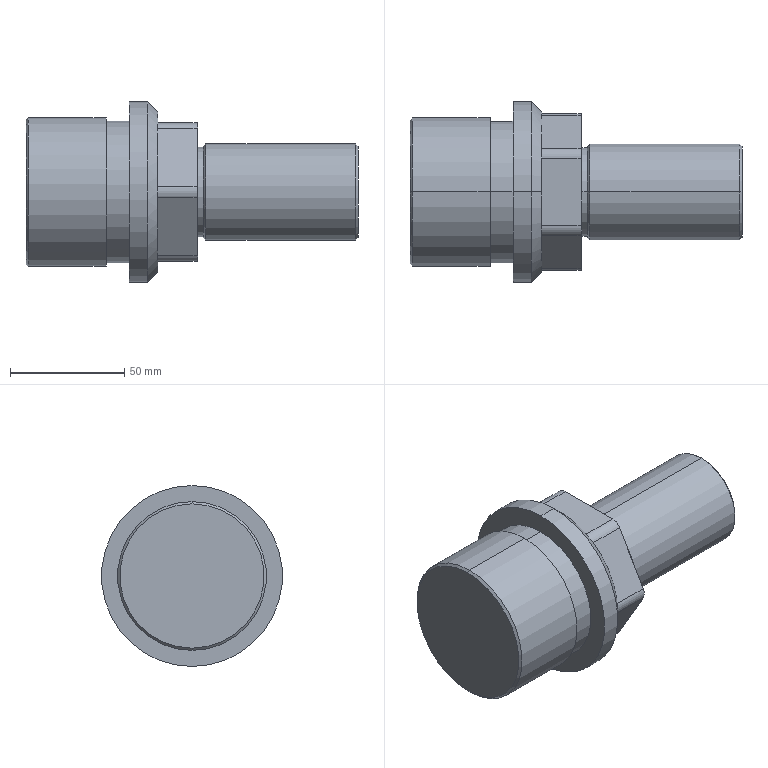Part | SolidWorks | features ICE 7, Chamfer 6, Draft 2, Extrusion 1, Fillet 1, MoveFace 1 | 1 solid | 49 faces | box 145 x 79 x 79 mm | volume 357004 mm3 | plane 19 | cylinder 16 | cone 14 | commonest cylinder face diameters 10 x6 39 x2 42 x2 62 x2 65 x2 79 x2
STEP:
#1=CARTESIAN_POINT('',(57.5,0.,-35.));
#2=VERTEX_POINT('',#1);
#3=CARTESIAN_POINT('',(57.5,0.,35.));
#4=VERTEX_POINT('',#3);
#5=CARTESIAN_POINT('',(57.5,0.,0.));
#6=DIRECTION('',(1.,0.,0.));
#7=DIRECTION('',(0.,0.,-1.));
#8=AXIS2_PLACEMENT_3D('',#5,#6,#7);
#9=CIRCLE('',#8,35.);
#10=EDGE_CURVE('',#2,#4,#9,.T.);
#11=ORIENTED_EDGE('',*,*,#10,.F.);
#12=CARTESIAN_POINT('',(53.,0.,-39.5));
#13=VERTEX_POINT('',#12);
#14=CARTESIAN_POINT('',(57.5,0.,-35.));
#15=DIRECTION('',(-0.7071,0.,-0.7071));
#16=VECTOR('',#15,1000.);
#17=LINE('',#14,#16);
#18=EDGE_CURVE('',#2,#13,#17,.T.);
#19=ORIENTED_EDGE('',*,*,#18,.T.);
#20=CARTESIAN_POINT('',(53.,0.,39.5));
#21=VERTEX_POINT('',#20);
#22=CARTESIAN_POINT('',(53.,0.,0.));
#23=DIRECTION('',(1.,0.,0.));
#24=DIRECTION('',(0.,0.,-1.));
#25=AXIS2_PLACEMENT_3D('',#22,#23,#24);
#26=CIRCLE('',#25,39.5);
#27=EDGE_CURVE('',#13,#21,#26,.T.);
#28=ORIENTED_EDGE('',*,*,#27,.T.);
#29=CARTESIAN_POINT('',(57.5,0.,35.));
#30=DIRECTION('',(-0.7071,0.,0.7071));
#31=VECTOR('',#30,1000.);
#32=LINE('',#29,#31);
#33=EDGE_CURVE('',#4,#21,#32,.T.);
#34=ORIENTED_EDGE('',*,*,#33,.F.);
#35=EDGE_LOOP('',(#11,#19,#28,#34));
#36=FACE_OUTER_BOUND('',#35,.T.);
#37=CARTESIAN_POINT('',(57.5,0.,0.));
#38=DIRECTION('',(-1.,0.,0.));
#39=DIRECTION('',(0.,0.,1.));
#40=AXIS2_PLACEMENT_3D('',#37,#38,#39);
#41=CONICAL_SURFACE('',#40,35.,0.7854);
#42=ADVANCED_FACE('',(#36),#41,.T.);
#43=CARTESIAN_POINT('',(77.5,0.,-19.5));
#44=VERTEX_POINT('',#43);
#45=CARTESIAN_POINT('',(77.5,0.,19.5));
#46=VERTEX_POINT('',#45);
#47=CARTESIAN_POINT('',(77.5,0.,0.));
#48=DIRECTION('',(1.,0.,0.));
#49=DIRECTION('',(0.,0.,-1.));
#50=AXIS2_PLACEMENT_3D('',#47,#48,#49);
#51=CIRCLE('',#50,19.5);
#52=EDGE_CURVE('',#44,#46,#51,.T.);
#53=ORIENTED_EDGE('',*,*,#52,.F.);
#54=CARTESIAN_POINT('',(75.,0.,-19.5));
#55=VERTEX_POINT('',#54);
#56=CARTESIAN_POINT('',(77.5,0.,-19.5));
#57=DIRECTION('',(-1.,0.,0.));
#58=VECTOR('',#57,1000.);
#59=LINE('',#56,#58);
#60=EDGE_CURVE('',#44,#55,#59,.T.);
#61=ORIENTED_EDGE('',*,*,#60,.T.);
#62=CARTESIAN_POINT('',(75.,0.,19.5));
#63=VERTEX_POINT('',#62);
#64=CARTESIAN_POINT('',(75.,0.,0.));
#65=DIRECTION('',(1.,0.,0.));
#66=DIRECTION('',(0.,0.,-1.));
#67=AXIS2_PLACEMENT_3D('',#64,#65,#66);
#68=CIRCLE('',#67,19.5);
#69=EDGE_CURVE('',#55,#63,#68,.T.);
#70=ORIENTED_EDGE('',*,*,#69,.T.);
#71=CARTESIAN_POINT('',(77.5,0.,19.5));
#72=DIRECTION('',(-1.,0.,0.));
#73=VECTOR('',#72,1000.);
#74=LINE('',#71,#73);
#75=EDGE_CURVE('',#46,#63,#74,.T.);
#76=ORIENTED_EDGE('',*,*,#75,.F.);
#77=EDGE_LOOP('',(#53,#61,#70,#76));
#78=FACE_OUTER_BOUND('',#77,.T.);
#79=CARTESIAN_POINT('',(77.5,0.,0.));
#80=DIRECTION('',(-1.,0.,0.));
#81=DIRECTION('',(0.,0.,1.));
#82=AXIS2_PLACEMENT_3D('',#79,#80,#81);
#83=CYLINDRICAL_SURFACE('',#82,19.5);
#84=ADVANCED_FACE('',(#78),#83,.T.);
#85=CARTESIAN_POINT('',(77.5,0.,20.));
#86=VERTEX_POINT('',#85);
#87=CARTESIAN_POINT('',(77.5,0.,-20.));
#88=VERTEX_POINT('',#87);
#89=CARTESIAN_POINT('',(77.5,0.,0.));
#90=DIRECTION('',(-1.,0.,0.));
#91=DIRECTION('',(0.,0.,-1.));
#92=AXIS2_PLACEMENT_3D('',#89,#90,#91);
#93=CIRCLE('',#92,20.);
#94=EDGE_CURVE('',#86,#88,#93,.T.);
#95=ORIENTED_EDGE('',*,*,#94,.F.);
#96=CARTESIAN_POINT('',(78.5,0.,21.));
#97=VERTEX_POINT('',#96);
#98=CARTESIAN_POINT('',(77.5,0.,20.));
#99=DIRECTION('',(0.7071,0.,0.7071));
#100=VECTOR('',#99,1000.);
#101=LINE('',#98,#100);
#102=EDGE_CURVE('',#86,#97,#101,.T.);
#103=ORIENTED_EDGE('',*,*,#102,.T.);
#104=CARTESIAN_POINT('',(78.5,0.,-21.));
#105=VERTEX_POINT('',#104);
#106=CARTESIAN_POINT('',(78.5,0.,0.));
#107=DIRECTION('',(1.,0.,0.));
#108=DIRECTION('',(0.,0.,-1.));
#109=AXIS2_PLACEMENT_3D('',#106,#107,#108);
#110=CIRCLE('',#109,21.);
#111=EDGE_CURVE('',#105,#97,#110,.T.);
#112=ORIENTED_EDGE('',*,*,#111,.F.);
#113=CARTESIAN_POINT('',(77.5,0.,-20.));
#114=DIRECTION('',(0.7071,0.,-0.7071));
#115=VECTOR('',#114,1000.);
#116=LINE('',#113,#115);
#117=EDGE_CURVE('',#88,#105,#116,.T.);
#118=ORIENTED_EDGE('',*,*,#117,.F.);
#119=EDGE_LOOP('',(#95,#103,#112,#118));
#120=FACE_OUTER_BOUND('',#119,.T.);
#121=CARTESIAN_POINT('',(77.5,0.,0.));
#122=DIRECTION('',(1.,0.,0.));
#123=DIRECTION('',(0.,0.,-1.));
#124=AXIS2_PLACEMENT_3D('',#121,#122,#123);
#125=CONICAL_SURFACE('',#124,20.,0.7854);
#126=ADVANCED_FACE('',(#120),#125,.T.);
#127=ORIENTED_EDGE('',*,*,#111,.T.);
#128=CARTESIAN_POINT('',(144.,0.,21.));
#129=VERTEX_POINT('',#128);
#130=CARTESIAN_POINT('',(75.,0.,21.));
#131=DIRECTION('',(1.,0.,0.));
#132=VECTOR('',#131,1000.);
#133=LINE('',#130,#132);
#134=EDGE_CURVE('',#97,#129,#133,.T.);
#135=ORIENTED_EDGE('',*,*,#134,.T.);
#136=CARTESIAN_POINT('',(144.,0.,-21.));
#137=VERTEX_POINT('',#136);
#138=CARTESIAN_POINT('',(144.,0.,0.));
#139=DIRECTION('',(-1.,0.,0.));
#140=DIRECTION('',(0.,0.,-1.));
#141=AXIS2_PLACEMENT_3D('',#138,#139,#140);
#142=CIRCLE('',#141,21.);
#143=EDGE_CURVE('',#129,#137,#142,.T.);
#144=ORIENTED_EDGE('',*,*,#143,.T.);
#145=CARTESIAN_POINT('',(75.,0.,-21.));
#146=DIRECTION('',(1.,0.,0.));
#147=VECTOR('',#146,1000.);
#148=LINE('',#145,#147);
#149=EDGE_CURVE('',#105,#137,#148,.T.);
#150=ORIENTED_EDGE('',*,*,#149,.F.);
#151=EDGE_LOOP('',(#127,#135,#144,#150));
#152=FACE_OUTER_BOUND('',#151,.T.);
#153=CARTESIAN_POINT('',(75.,0.,0.));
#154=DIRECTION('',(1.,0.,0.));
#155=DIRECTION('',(0.,0.,-1.));
#156=AXIS2_PLACEMENT_3D('',#153,#154,#155);
#157=CYLINDRICAL_SURFACE('',#156,21.);
#158=ADVANCED_FACE('',(#152),#157,.T.);
#159=CARTESIAN_POINT('',(145.,0.,-20.));
#160=VERTEX_POINT('',#159);
#161=CARTESIAN_POINT('',(145.,0.,20.));
#162=VERTEX_POINT('',#161);
#163=CARTESIAN_POINT('',(145.,0.,0.));
#164=DIRECTION('',(1.,0.,0.));
#165=DIRECTION('',(0.,0.,-1.));
#166=AXIS2_PLACEMENT_3D('',#163,#164,#165);
#167=CIRCLE('',#166,20.);
#168=EDGE_CURVE('',#160,#162,#167,.T.);
#169=ORIENTED_EDGE('',*,*,#168,.F.);
#170=CARTESIAN_POINT('',(145.,0.,-20.));
#171=DIRECTION('',(-0.7071,0.,-0.7071));
#172=VECTOR('',#171,1000.);
#173=LINE('',#170,#172);
#174=EDGE_CURVE('',#160,#137,#173,.T.);
#175=ORIENTED_EDGE('',*,*,#174,.T.);
#176=ORIENTED_EDGE('',*,*,#143,.F.);
#177=CARTESIAN_POINT('',(145.,0.,20.));
#178=DIRECTION('',(-0.7071,0.,0.7071));
#179=VECTOR('',#178,1000.);
#180=LINE('',#177,#179);
#181=EDGE_CURVE('',#162,#129,#180,.T.);
#182=ORIENTED_EDGE('',*,*,#181,.F.);
#183=EDGE_LOOP('',(#169,#175,#176,#182));
#184=FACE_OUTER_BOUND('',#183,.T.);
#185=CARTESIAN_POINT('',(145.,0.,0.));
#186=DIRECTION('',(-1.,0.,0.));
#187=DIRECTION('',(0.,0.,1.));
#188=AXIS2_PLACEMENT_3D('',#185,#186,#187);
#189=CONICAL_SURFACE('',#188,20.,0.7854);
#190=ADVANCED_FACE('',(#184),#189,.T.);
#191=CARTESIAN_POINT('',(0.,0.,31.5));
#192=VERTEX_POINT('',#191);
#193=CARTESIAN_POINT('',(0.,0.,-31.5));
#194=VERTEX_POINT('',#193);
#195=CARTESIAN_POINT('',(0.,0.,0.));
#196=DIRECTION('',(-1.,0.,0.));
#197=DIRECTION('',(0.,0.,-1.));
#198=AXIS2_PLACEMENT_3D('',#195,#196,#197);
#199=CIRCLE('',#198,31.5);
#200=EDGE_CURVE('',#192,#194,#199,.T.);
#201=ORIENTED_EDGE('',*,*,#200,.F.);
#202=CARTESIAN_POINT('',(1.,0.,32.5));
#203=VERTEX_POINT('',#202);
#204=CARTESIAN_POINT('',(0.,0.,31.5));
#205=DIRECTION('',(0.7071,0.,0.7071));
#206=VECTOR('',#205,1000.);
#207=LINE('',#204,#206);
#208=EDGE_CURVE('',#192,#203,#207,.T.);
#209=ORIENTED_EDGE('',*,*,#208,.T.);
#210=CARTESIAN_POINT('',(1.,0.,-32.5));
#211=VERTEX_POINT('',#210);
#212=CARTESIAN_POINT('',(1.,0.,0.));
#213=DIRECTION('',(1.,0.,0.));
#214=DIRECTION('',(0.,0.,-1.));
#215=AXIS2_PLACEMENT_3D('',#212,#213,#214);
#216=CIRCLE('',#215,32.5);
#217=EDGE_CURVE('',#211,#203,#216,.T.);
#218=ORIENTED_EDGE('',*,*,#217,.F.);
#219=CARTESIAN_POINT('',(0.,0.,-31.5));
#220=DIRECTION('',(0.7071,0.,-0.7071));
#221=VECTOR('',#220,1000.);
#222=LINE('',#219,#221);
#223=EDGE_CURVE('',#194,#211,#222,.T.);
#224=ORIENTED_EDGE('',*,*,#223,.F.);
#225=EDGE_LOOP('',(#201,#209,#218,#224));
#226=FACE_OUTER_BOUND('',#225,.T.);
#227=CARTESIAN_POINT('',(0.,0.,0.));
#228=DIRECTION('',(1.,0.,0.));
#229=DIRECTION('',(0.,0.,-1.));
#230=AXIS2_PLACEMENT_3D('',#227,#228,#229);
#231=CONICAL_SURFACE('',#230,31.5,0.7854);
#232=ADVANCED_FACE('',(#226),#231,.T.);
#233=CARTESIAN_POINT('',(35.,0.,-32.5));
#234=VERTEX_POINT('',#233);
#235=CARTESIAN_POINT('',(35.,0.,32.5));
#236=VERTEX_POINT('',#235);
#237=CARTESIAN_POINT('',(35.,0.,0.));
#238=DIRECTION('',(1.,0.,0.));
#239=DIRECTION('',(0.,0.,1.));
#240=AXIS2_PLACEMENT_3D('',#237,#238,#239);
#241=CIRCLE('',#240,32.5);
#242=EDGE_CURVE('',#234,#236,#241,.T.);
#243=ORIENTED_EDGE('',*,*,#242,.F.);
#244=CARTESIAN_POINT('',(45.,0.,-32.5));
#245=DIRECTION('',(-1.,0.,0.));
#246=VECTOR('',#245,1000.);
#247=LINE('',#244,#246);
#248=EDGE_CURVE('',#234,#211,#247,.T.);
#249=ORIENTED_EDGE('',*,*,#248,.T.);
#250=ORIENTED_EDGE('',*,*,#217,.T.);
#251=CARTESIAN_POINT('',(45.,0.,32.5));
#252=DIRECTION('',(-1.,0.,0.));
#253=VECTOR('',#252,1000.);
#254=LINE('',#251,#253);
#255=EDGE_CURVE('',#236,#203,#254,.T.);
#256=ORIENTED_EDGE('',*,*,#255,.F.);
#257=EDGE_LOOP('',(#243,#249,#250,#256));
#258=FACE_OUTER_BOUND('',#257,.T.);
#259=CARTESIAN_POINT('',(45.,0.,0.));
#260=DIRECTION('',(-1.,0.,0.));
#261=DIRECTION('',(0.,0.,1.));
#262=AXIS2_PLACEMENT_3D('',#259,#260,#261);
#263=CYLINDRICAL_SURFACE('',#262,32.5);
#264=ADVANCED_FACE('',(#258),#263,.T.);
#265=CARTESIAN_POINT('',(35.,0.,31.));
#266=VERTEX_POINT('',#265);
#267=CARTESIAN_POINT('',(35.,0.,-31.));
#268=VERTEX_POINT('',#267);
#269=CARTESIAN_POINT('',(35.,0.,0.));
#270=DIRECTION('',(-1.,0.,0.));
#271=DIRECTION('',(0.,0.,1.));
#272=AXIS2_PLACEMENT_3D('',#269,#270,#271);
#273=CIRCLE('',#272,31.);
#274=EDGE_CURVE('',#266,#268,#273,.T.);
#275=ORIENTED_EDGE('',*,*,#274,.F.);
#276=CARTESIAN_POINT('',(45.,0.,31.));
#277=VERTEX_POINT('',#276);
#278=CARTESIAN_POINT('',(35.,0.,31.));
#279=DIRECTION('',(1.,0.,0.));
#280=VECTOR('',#279,1000.);
#281=LINE('',#278,#280);
#282=EDGE_CURVE('',#266,#277,#281,.T.);
#283=ORIENTED_EDGE('',*,*,#282,.T.);
#284=CARTESIAN_POINT('',(45.,0.,-31.));
#285=VERTEX_POINT('',#284);
#286=CARTESIAN_POINT('',(45.,0.,0.));
#287=DIRECTION('',(-1.,0.,0.));
#288=DIRECTION('',(0.,0.,1.));
#289=AXIS2_PLACEMENT_3D('',#286,#287,#288);
#290=CIRCLE('',#289,31.);
#291=EDGE_CURVE('',#277,#285,#290,.T.);
#292=ORIENTED_EDGE('',*,*,#291,.T.);
#293=CARTESIAN_POINT('',(35.,0.,-31.));
#294=DIRECTION('',(1.,0.,0.));
#295=VECTOR('',#294,1000.);
#296=LINE('',#293,#295);
#297=EDGE_CURVE('',#268,#285,#296,.T.);
#298=ORIENTED_EDGE('',*,*,#297,.F.);
#299=EDGE_LOOP('',(#275,#283,#292,#298));
#300=FACE_OUTER_BOUND('',#299,.T.);
#301=CARTESIAN_POINT('',(35.,0.,0.));
#302=DIRECTION('',(1.,0.,0.));
#303=DIRECTION('',(0.,0.,-1.));
#304=AXIS2_PLACEMENT_3D('',#301,#302,#303);
#305=CYLINDRICAL_SURFACE('',#304,31.);
#306=ADVANCED_FACE('',(#300),#305,.T.);
#307=ORIENTED_EDGE('',*,*,#27,.F.);
#308=CARTESIAN_POINT('',(45.,0.,-39.5));
#309=VERTEX_POINT('',#308);
#310=CARTESIAN_POINT('',(145.,0.,-39.5));
#311=DIRECTION('',(-1.,0.,0.));
#312=VECTOR('',#311,1000.);
#313=LINE('',#310,#312);
#314=EDGE_CURVE('',#13,#309,#313,.T.);
#315=ORIENTED_EDGE('',*,*,#314,.T.);
#316=CARTESIAN_POINT('',(45.,0.,39.5));
#317=VERTEX_POINT('',#316);
#318=CARTESIAN_POINT('',(45.,0.,0.));
#319=DIRECTION('',(-1.,0.,0.));
#320=DIRECTION('',(0.,0.,1.));
#321=AXIS2_PLACEMENT_3D('',#318,#319,#320);
#322=CIRCLE('',#321,39.5);
#323=EDGE_CURVE('',#317,#309,#322,.T.);
#324=ORIENTED_EDGE('',*,*,#323,.F.);
#325=CARTESIAN_POINT('',(145.,0.,39.5));
#326=DIRECTION('',(-1.,0.,0.));
#327=VECTOR('',#326,1000.);
#328=LINE('',#325,#327);
#329=EDGE_CURVE('',#21,#317,#328,.T.);
#330=ORIENTED_EDGE('',*,*,#329,.F.);
#331=EDGE_LOOP('',(#307,#315,#324,#330));
#332=FACE_OUTER_BOUND('',#331,.T.);
#333=CARTESIAN_POINT('',(145.,0.,0.));
#334=DIRECTION('',(-1.,0.,0.));
#335=DIRECTION('',(0.,0.,1.));
#336=AXIS2_PLACEMENT_3D('',#333,#334,#335);
#337=CYLINDRICAL_SURFACE('',#336,39.5);
#338=ADVANCED_FACE('',(#332),#337,.T.);
#339=ORIENTED_EDGE('',*,*,#314,.F.);
#340=CARTESIAN_POINT('',(53.,0.,0.));
#341=DIRECTION('',(1.,0.,0.));
#342=DIRECTION('',(0.,0.,-1.));
#343=AXIS2_PLACEMENT_3D('',#340,#341,#342);
#344=CIRCLE('',#343,39.5);
#345=EDGE_CURVE('',#21,#13,#344,.T.);
#346=ORIENTED_EDGE('',*,*,#345,.F.);
#347=ORIENTED_EDGE('',*,*,#329,.T.);
#348=CARTESIAN_POINT('',(45.,0.,0.));
#349=DIRECTION('',(-1.,0.,0.));
#350=DIRECTION('',(0.,0.,1.));
#351=AXIS2_PLACEMENT_3D('',#348,#349,#350);
#352=CIRCLE('',#351,39.5);
#353=EDGE_CURVE('',#309,#317,#352,.T.);
#354=ORIENTED_EDGE('',*,*,#353,.F.);
#355=EDGE_LOOP('',(#339,#346,#347,#354));
#356=FACE_OUTER_BOUND('',#355,.T.);
#357=CARTESIAN_POINT('',(145.,0.,0.));
#358=DIRECTION('',(-1.,0.,0.));
#359=DIRECTION('',(0.,0.,1.));
#360=AXIS2_PLACEMENT_3D('',#357,#358,#359);
#361=CYLINDRICAL_SURFACE('',#360,39.5);
#362=ADVANCED_FACE('',(#356),#361,.T.);
#363=ORIENTED_EDGE('',*,*,#323,.T.);
#364=ORIENTED_EDGE('',*,*,#353,.T.);
#365=EDGE_LOOP('',(#363,#364));
#366=FACE_OUTER_BOUND('',#365,.T.);
#367=CARTESIAN_POINT('',(45.,0.,0.));
#368=DIRECTION('',(-1.,0.,0.));
#369=DIRECTION('',(0.,0.,1.));
#370=AXIS2_PLACEMENT_3D('',#367,#368,#369);
#371=CIRCLE('',#370,31.);
#372=EDGE_CURVE('',#285,#277,#371,.T.);
#373=ORIENTED_EDGE('',*,*,#372,.F.);
#374=ORIENTED_EDGE('',*,*,#291,.F.);
#375=EDGE_LOOP('',(#373,#374));
#376=FACE_BOUND('',#375,.T.);
#377=CARTESIAN_POINT('',(45.,0.,0.));
#378=DIRECTION('',(-1.,0.,0.));
#379=DIRECTION('',(0.,0.,1.));
#380=AXIS2_PLACEMENT_3D('',#377,#378,#379);
#381=PLANE('',#380);
#382=ADVANCED_FACE('',(#366,#376),#381,.T.);
#383=CARTESIAN_POINT('',(35.,0.,0.));
#384=DIRECTION('',(1.,0.,0.));
#385=DIRECTION('',(0.,0.,1.));
#386=AXIS2_PLACEMENT_3D('',#383,#384,#385);
#387=CIRCLE('',#386,32.5);
#388=EDGE_CURVE('',#236,#234,#387,.T.);
#389=ORIENTED_EDGE('',*,*,#388,.T.);
#390=ORIENTED_EDGE('',*,*,#242,.T.);
#391=EDGE_LOOP('',(#389,#390));
#392=FACE_OUTER_BOUND('',#391,.T.);
#393=CARTESIAN_POINT('',(35.,0.,0.));
#394=DIRECTION('',(-1.,0.,0.));
#395=DIRECTION('',(0.,0.,1.));
#396=AXIS2_PLACEMENT_3D('',#393,#394,#395);
#397=CIRCLE('',#396,31.);
#398=EDGE_CURVE('',#268,#266,#397,.T.);
#399=ORIENTED_EDGE('',*,*,#398,.T.);
#400=ORIENTED_EDGE('',*,*,#274,.T.);
#401=EDGE_LOOP('',(#399,#400));
#402=FACE_BOUND('',#401,.T.);
#403=CARTESIAN_POINT('',(35.,0.,0.));
#404=DIRECTION('',(-1.,0.,0.));
#405=DIRECTION('',(0.,0.,1.));
#406=AXIS2_PLACEMENT_3D('',#403,#404,#405);
#407=PLANE('',#406);
#408=ADVANCED_FACE('',(#392,#402),#407,.F.);
#409=ORIENTED_EDGE('',*,*,#282,.F.);
#410=ORIENTED_EDGE('',*,*,#398,.F.);
#411=ORIENTED_EDGE('',*,*,#297,.T.);
#412=ORIENTED_EDGE('',*,*,#372,.T.);
#413=EDGE_LOOP('',(#409,#410,#411,#412));
#414=FACE_OUTER_BOUND('',#413,.T.);
#415=CARTESIAN_POINT('',(35.,0.,0.));
#416=DIRECTION('',(1.,0.,0.));
#417=DIRECTION('',(0.,0.,-1.));
#418=AXIS2_PLACEMENT_3D('',#415,#416,#417);
#419=CYLINDRICAL_SURFACE('',#418,31.);
#420=ADVANCED_FACE('',(#414),#419,.T.);
#421=CARTESIAN_POINT('',(0.,0.,0.));
#422=DIRECTION('',(-1.,0.,0.));
#423=DIRECTION('',(0.,0.,-1.));
#424=AXIS2_PLACEMENT_3D('',#421,#422,#423);
#425=CIRCLE('',#424,31.5);
#426=EDGE_CURVE('',#194,#192,#425,.T.);
#427=ORIENTED_EDGE('',*,*,#426,.T.);
#428=ORIENTED_EDGE('',*,*,#200,.T.);
#429=EDGE_LOOP('',(#427,#428));
#430=FACE_OUTER_BOUND('',#429,.T.);
#431=CARTESIAN_POINT('',(0.,0.,0.));
#432=DIRECTION('',(1.,0.,0.));
#433=DIRECTION('',(0.,0.,-1.));
#434=AXIS2_PLACEMENT_3D('',#431,#432,#433);
#435=PLANE('',#434);
#436=ADVANCED_FACE('',(#430),#435,.F.);
#437=ORIENTED_EDGE('',*,*,#248,.F.);
#438=ORIENTED_EDGE('',*,*,#388,.F.);
#439=ORIENTED_EDGE('',*,*,#255,.T.);
#440=CARTESIAN_POINT('',(1.,0.,0.));
#441=DIRECTION('',(1.,0.,0.));
#442=DIRECTION('',(0.,0.,-1.));
#443=AXIS2_PLACEMENT_3D('',#440,#441,#442);
#444=CIRCLE('',#443,32.5);
#445=EDGE_CURVE('',#203,#211,#444,.T.);
#446=ORIENTED_EDGE('',*,*,#445,.T.);
#447=EDGE_LOOP('',(#437,#438,#439,#446));
#448=FACE_OUTER_BOUND('',#447,.T.);
#449=CARTESIAN_POINT('',(45.,0.,0.));
#450=DIRECTION('',(-1.,0.,0.));
#451=DIRECTION('',(0.,0.,1.));
#452=AXIS2_PLACEMENT_3D('',#449,#450,#451);
#453=CYLINDRICAL_SURFACE('',#452,32.5);
#454=ADVANCED_FACE('',(#448),#453,.T.);
#455=ORIENTED_EDGE('',*,*,#208,.F.);
#456=ORIENTED_EDGE('',*,*,#426,.F.);
#457=ORIENTED_EDGE('',*,*,#223,.T.);
#458=ORIENTED_EDGE('',*,*,#445,.F.);
#459=EDGE_LOOP('',(#455,#456,#457,#458));
#460=FACE_OUTER_BOUND('',#459,.T.);
#461=CARTESIAN_POINT('',(0.,0.,0.));
#462=DIRECTION('',(1.,0.,0.));
#463=DIRECTION('',(0.,0.,-1.));
#464=AXIS2_PLACEMENT_3D('',#461,#462,#463);
#465=CONICAL_SURFACE('',#464,31.5,0.7854);
#466=ADVANCED_FACE('',(#460),#465,.T.);
#467=CARTESIAN_POINT('',(57.5,-18.943,-27.811));
#468=VERTEX_POINT('',#467);
#469=CARTESIAN_POINT('',(57.5,-33.557,-2.5));
#470=VERTEX_POINT('',#469);
#471=CARTESIAN_POINT('',(57.5,-35.,0.));
#472=DIRECTION('',(0.,-0.5,0.866));
#473=VECTOR('',#472,1000.);
#474=LINE('',#471,#473);
#475=EDGE_CURVE('',#468,#470,#474,.T.);
#476=ORIENTED_EDGE('',*,*,#475,.T.);
#477=CARTESIAN_POINT('',(57.5,-33.557,2.5));
#478=VERTEX_POINT('',#477);
#479=CARTESIAN_POINT('',(57.5,-29.226,0.));
#480=DIRECTION('',(-1.,0.,0.));
#481=DIRECTION('',(0.,0.,-1.));
#482=AXIS2_PLACEMENT_3D('',#479,#480,#481);
#483=CIRCLE('',#482,5.);
#484=EDGE_CURVE('',#470,#478,#483,.T.);
#485=ORIENTED_EDGE('',*,*,#484,.T.);
#486=CARTESIAN_POINT('',(57.5,-18.943,27.811));
#487=VERTEX_POINT('',#486);
#488=CARTESIAN_POINT('',(57.5,-17.5,30.311));
#489=DIRECTION('',(0.,0.5,0.866));
#490=VECTOR('',#489,1000.);
#491=LINE('',#488,#490);
#492=EDGE_CURVE('',#478,#487,#491,.T.);
#493=ORIENTED_EDGE('',*,*,#492,.T.);
#494=CARTESIAN_POINT('',(57.5,-14.613,30.311));
#495=VERTEX_POINT('',#494);
#496=CARTESIAN_POINT('',(57.5,-14.613,25.311));
#497=DIRECTION('',(-1.,0.,0.));
#498=DIRECTION('',(0.,0.,-1.));
#499=AXIS2_PLACEMENT_3D('',#496,#497,#498);
#500=CIRCLE('',#499,5.);
#501=EDGE_CURVE('',#487,#495,#500,.T.);
#502=ORIENTED_EDGE('',*,*,#501,.T.);
#503=CARTESIAN_POINT('',(57.5,14.613,30.311));
#504=VERTEX_POINT('',#503);
#505=CARTESIAN_POINT('',(57.5,17.5,30.311));
#506=DIRECTION('',(0.,1.,0.));
#507=VECTOR('',#506,1000.);
#508=LINE('',#505,#507);
#509=EDGE_CURVE('',#495,#504,#508,.T.);
#510=ORIENTED_EDGE('',*,*,#509,.T.);
#511=CARTESIAN_POINT('',(57.5,18.943,27.811));
#512=VERTEX_POINT('',#511);
#513=CARTESIAN_POINT('',(57.5,14.613,25.311));
#514=DIRECTION('',(-1.,0.,0.));
#515=DIRECTION('',(0.,0.,-1.));
#516=AXIS2_PLACEMENT_3D('',#513,#514,#515);
#517=CIRCLE('',#516,5.);
#518=EDGE_CURVE('',#504,#512,#517,.T.);
#519=ORIENTED_EDGE('',*,*,#518,.T.);
#520=CARTESIAN_POINT('',(57.5,33.557,2.5));
#521=VERTEX_POINT('',#520);
#522=CARTESIAN_POINT('',(57.5,35.,0.));
#523=DIRECTION('',(0.,0.5,-0.866));
#524=VECTOR('',#523,1000.);
#525=LINE('',#522,#524);
#526=EDGE_CURVE('',#512,#521,#525,.T.);
#527=ORIENTED_EDGE('',*,*,#526,.T.);
#528=CARTESIAN_POINT('',(57.5,33.557,-2.5));
#529=VERTEX_POINT('',#528);
#530=CARTESIAN_POINT('',(57.5,29.226,0.));
#531=DIRECTION('',(-1.,0.,0.));
#532=DIRECTION('',(0.,0.,-1.));
#533=AXIS2_PLACEMENT_3D('',#530,#531,#532);
#534=CIRCLE('',#533,5.);
#535=EDGE_CURVE('',#521,#529,#534,.T.);
#536=ORIENTED_EDGE('',*,*,#535,.T.);
#537=CARTESIAN_POINT('',(57.5,18.943,-27.811));
#538=VERTEX_POINT('',#537);
#539=CARTESIAN_POINT('',(57.5,17.5,-30.311));
#540=DIRECTION('',(0.,-0.5,-0.866));
#541=VECTOR('',#540,1000.);
#542=LINE('',#539,#541);
#543=EDGE_CURVE('',#529,#538,#542,.T.);
#544=ORIENTED_EDGE('',*,*,#543,.T.);
#545=CARTESIAN_POINT('',(57.5,14.613,-30.311));
#546=VERTEX_POINT('',#545);
#547=CARTESIAN_POINT('',(57.5,14.613,-25.311));
#548=DIRECTION('',(-1.,0.,0.));
#549=DIRECTION('',(0.,0.,-1.));
#550=AXIS2_PLACEMENT_3D('',#547,#548,#549);
#551=CIRCLE('',#550,5.);
#552=EDGE_CURVE('',#538,#546,#551,.T.);
#553=ORIENTED_EDGE('',*,*,#552,.T.);
#554=CARTESIAN_POINT('',(57.5,-14.613,-30.311));
#555=VERTEX_POINT('',#554);
#556=CARTESIAN_POINT('',(57.5,-17.5,-30.311));
#557=DIRECTION('',(0.,-1.,0.));
#558=VECTOR('',#557,1000.);
#559=LINE('',#556,#558);
#560=EDGE_CURVE('',#546,#555,#559,.T.);
#561=ORIENTED_EDGE('',*,*,#560,.T.);
#562=CARTESIAN_POINT('',(57.5,-14.613,-25.311));
#563=DIRECTION('',(-1.,0.,0.));
#564=DIRECTION('',(0.,0.,-1.));
#565=AXIS2_PLACEMENT_3D('',#562,#563,#564);
#566=CIRCLE('',#565,5.);
#567=EDGE_CURVE('',#555,#468,#566,.T.);
#568=ORIENTED_EDGE('',*,*,#567,.T.);
#569=EDGE_LOOP('',(#476,#485,#493,#502,#510,#519,#527,#536,#544,#553,#561,#568));
#570=FACE_BOUND('',#569,.T.);
#571=CARTESIAN_POINT('',(57.5,0.,0.));
#572=DIRECTION('',(1.,0.,0.));
#573=DIRECTION('',(0.,0.,-1.));
#574=AXIS2_PLACEMENT_3D('',#571,#572,#573);
#575=CIRCLE('',#574,35.);
#576=EDGE_CURVE('',#4,#2,#575,.T.);
#577=ORIENTED_EDGE('',*,*,#576,.T.);
#578=ORIENTED_EDGE('',*,*,#10,.T.);
#579=EDGE_LOOP('',(#577,#578));
#580=FACE_OUTER_BOUND('',#579,.T.);
#581=CARTESIAN_POINT('',(57.5,0.,0.));
#582=DIRECTION('',(1.,0.,0.));
#583=DIRECTION('',(0.,0.,-1.));
#584=AXIS2_PLACEMENT_3D('',#581,#582,#583);
#585=PLANE('',#584);
#586=ADVANCED_FACE('',(#570,#580),#585,.T.);
#587=CARTESIAN_POINT('',(145.,0.,0.));
#588=DIRECTION('',(1.,0.,0.));
#589=DIRECTION('',(0.,0.,-1.));
#590=AXIS2_PLACEMENT_3D('',#587,#588,#589);
#591=CIRCLE('',#590,20.);
#592=EDGE_CURVE('',#162,#160,#591,.T.);
#593=ORIENTED_EDGE('',*,*,#592,.T.);
#594=ORIENTED_EDGE('',*,*,#168,.T.);
#595=EDGE_LOOP('',(#593,#594));
#596=FACE_OUTER_BOUND('',#595,.T.);
#597=CARTESIAN_POINT('',(145.,0.,0.));
#598=DIRECTION('',(1.,0.,0.));
#599=DIRECTION('',(0.,0.,-1.));
#600=AXIS2_PLACEMENT_3D('',#597,#598,#599);
#601=PLANE('',#600);
#602=ADVANCED_FACE('',(#596),#601,.T.);
#603=ORIENTED_EDGE('',*,*,#174,.F.);
#604=ORIENTED_EDGE('',*,*,#592,.F.);
#605=ORIENTED_EDGE('',*,*,#181,.T.);
#606=CARTESIAN_POINT('',(144.,0.,0.));
#607=DIRECTION('',(-1.,0.,0.));
#608=DIRECTION('',(0.,0.,-1.));
#609=AXIS2_PLACEMENT_3D('',#606,#607,#608);
#610=CIRCLE('',#609,21.);
#611=EDGE_CURVE('',#137,#129,#610,.T.);
#612=ORIENTED_EDGE('',*,*,#611,.F.);
#613=EDGE_LOOP('',(#603,#604,#605,#612));
#614=FACE_OUTER_BOUND('',#613,.T.);
#615=CARTESIAN_POINT('',(145.,0.,0.));
#616=DIRECTION('',(-1.,0.,0.));
#617=DIRECTION('',(0.,0.,1.));
#618=AXIS2_PLACEMENT_3D('',#615,#616,#617);
#619=CONICAL_SURFACE('',#618,20.,0.7854);
#620=ADVANCED_FACE('',(#614),#619,.T.);
#621=ORIENTED_EDGE('',*,*,#134,.F.);
#622=CARTESIAN_POINT('',(78.5,0.,0.));
#623=DIRECTION('',(1.,0.,0.));
#624=DIRECTION('',(0.,0.,-1.));
#625=AXIS2_PLACEMENT_3D('',#622,#623,#624);
#626=CIRCLE('',#625,21.);
#627=EDGE_CURVE('',#97,#105,#626,.T.);
#628=ORIENTED_EDGE('',*,*,#627,.T.);
#629=ORIENTED_EDGE('',*,*,#149,.T.);
#630=ORIENTED_EDGE('',*,*,#611,.T.);
#631=EDGE_LOOP('',(#621,#628,#629,#630));
#632=FACE_OUTER_BOUND('',#631,.T.);
#633=CARTESIAN_POINT('',(75.,0.,0.));
#634=DIRECTION('',(1.,0.,0.));
#635=DIRECTION('',(0.,0.,-1.));
#636=AXIS2_PLACEMENT_3D('',#633,#634,#635);
#637=CYLINDRICAL_SURFACE('',#636,21.);
#638=ADVANCED_FACE('',(#632),#637,.T.);
#639=ORIENTED_EDGE('',*,*,#102,.F.);
#640=CARTESIAN_POINT('',(77.5,0.,0.));
#641=DIRECTION('',(-1.,0.,0.));
#642=DIRECTION('',(0.,0.,-1.));
#643=AXIS2_PLACEMENT_3D('',#640,#641,#642);
#644=CIRCLE('',#643,20.);
#645=EDGE_CURVE('',#88,#86,#644,.T.);
#646=ORIENTED_EDGE('',*,*,#645,.F.);
#647=ORIENTED_EDGE('',*,*,#117,.T.);
#648=ORIENTED_EDGE('',*,*,#627,.F.);
#649=EDGE_LOOP('',(#639,#646,#647,#648));
#650=FACE_OUTER_BOUND('',#649,.T.);
#651=CARTESIAN_POINT('',(77.5,0.,0.));
#652=DIRECTION('',(1.,0.,0.));
#653=DIRECTION('',(0.,0.,-1.));
#654=AXIS2_PLACEMENT_3D('',#651,#652,#653);
#655=CONICAL_SURFACE('',#654,20.,0.7854);
#656=ADVANCED_FACE('',(#650),#655,.T.);
#657=ORIENTED_EDGE('',*,*,#645,.T.);
#658=ORIENTED_EDGE('',*,*,#94,.T.);
#659=EDGE_LOOP('',(#657,#658));
#660=FACE_OUTER_BOUND('',#659,.T.);
#661=CARTESIAN_POINT('',(77.5,0.,0.));
#662=DIRECTION('',(1.,0.,0.));
#663=DIRECTION('',(0.,0.,-1.));
#664=AXIS2_PLACEMENT_3D('',#661,#662,#663);
#665=CIRCLE('',#664,19.5);
#666=EDGE_CURVE('',#46,#44,#665,.T.);
#667=ORIENTED_EDGE('',*,*,#666,.T.);
#668=ORIENTED_EDGE('',*,*,#52,.T.);
#669=EDGE_LOOP('',(#667,#668));
#670=FACE_BOUND('',#669,.T.);
#671=CARTESIAN_POINT('',(77.5,0.,0.));
#672=DIRECTION('',(1.,0.,0.));
#673=DIRECTION('',(0.,0.,-1.));
#674=AXIS2_PLACEMENT_3D('',#671,#672,#673);
#675=PLANE('',#674);
#676=ADVANCED_FACE('',(#660,#670),#675,.F.);
#677=ORIENTED_EDGE('',*,*,#60,.F.);
#678=ORIENTED_EDGE('',*,*,#666,.F.);
#679=ORIENTED_EDGE('',*,*,#75,.T.);
#680=CARTESIAN_POINT('',(75.,0.,0.));
#681=DIRECTION('',(1.,0.,0.));
#682=DIRECTION('',(0.,0.,-1.));
#683=AXIS2_PLACEMENT_3D('',#680,#681,#682);
#684=CIRCLE('',#683,19.5);
#685=EDGE_CURVE('',#63,#55,#684,.T.);
#686=ORIENTED_EDGE('',*,*,#685,.T.);
#687=EDGE_LOOP('',(#677,#678,#679,#686));
#688=FACE_OUTER_BOUND('',#687,.T.);
#689=CARTESIAN_POINT('',(77.5,0.,0.));
#690=DIRECTION('',(-1.,0.,0.));
#691=DIRECTION('',(0.,0.,1.));
#692=AXIS2_PLACEMENT_3D('',#689,#690,#691);
#693=CYLINDRICAL_SURFACE('',#692,19.5);
#694=ADVANCED_FACE('',(#688),#693,.T.);
#695=CARTESIAN_POINT('',(75.,-18.684,-27.661));
#696=VERTEX_POINT('',#695);
#697=CARTESIAN_POINT('',(75.,-14.613,-30.011));
#698=VERTEX_POINT('',#697);
#699=CARTESIAN_POINT('',(75.,-14.613,-25.311));
#700=DIRECTION('',(1.,0.,0.));
#701=DIRECTION('',(0.,0.,-1.));
#702=AXIS2_PLACEMENT_3D('',#699,#700,#701);
#703=CIRCLE('',#702,4.7);
#704=EDGE_CURVE('',#696,#698,#703,.T.);
#705=ORIENTED_EDGE('',*,*,#704,.T.);
#706=CARTESIAN_POINT('',(75.,14.613,-30.011));
#707=VERTEX_POINT('',#706);
#708=CARTESIAN_POINT('',(75.,0.,-30.011));
#709=DIRECTION('',(0.,1.,0.));
#710=VECTOR('',#709,1000.);
#711=LINE('',#708,#710);
#712=EDGE_CURVE('',#698,#707,#711,.T.);
#713=ORIENTED_EDGE('',*,*,#712,.T.);
#714=CARTESIAN_POINT('',(75.,18.684,-27.661));
#715=VERTEX_POINT('',#714);
#716=CARTESIAN_POINT('',(75.,14.613,-25.311));
#717=DIRECTION('',(1.,0.,0.));
#718=DIRECTION('',(0.,0.,-1.));
#719=AXIS2_PLACEMENT_3D('',#716,#717,#718);
#720=CIRCLE('',#719,4.7);
#721=EDGE_CURVE('',#707,#715,#720,.T.);
#722=ORIENTED_EDGE('',*,*,#721,.T.);
#723=CARTESIAN_POINT('',(75.,33.297,-2.35));
#724=VERTEX_POINT('',#723);
#725=CARTESIAN_POINT('',(75.,25.99,-15.005));
#726=DIRECTION('',(0.,0.5,0.866));
#727=VECTOR('',#726,1000.);
#728=LINE('',#725,#727);
#729=EDGE_CURVE('',#715,#724,#728,.T.);
#730=ORIENTED_EDGE('',*,*,#729,.T.);
#731=CARTESIAN_POINT('',(75.,33.297,2.35));
#732=VERTEX_POINT('',#731);
#733=CARTESIAN_POINT('',(75.,29.226,0.));
#734=DIRECTION('',(1.,0.,0.));
#735=DIRECTION('',(0.,0.,-1.));
#736=AXIS2_PLACEMENT_3D('',#733,#734,#735);
#737=CIRCLE('',#736,4.7);
#738=EDGE_CURVE('',#724,#732,#737,.T.);
#739=ORIENTED_EDGE('',*,*,#738,.T.);
#740=CARTESIAN_POINT('',(75.,18.684,27.661));
#741=VERTEX_POINT('',#740);
#742=CARTESIAN_POINT('',(75.,25.99,15.005));
#743=DIRECTION('',(0.,-0.5,0.866));
#744=VECTOR('',#743,1000.);
#745=LINE('',#742,#744);
#746=EDGE_CURVE('',#732,#741,#745,.T.);
#747=ORIENTED_EDGE('',*,*,#746,.T.);
#748=CARTESIAN_POINT('',(75.,14.613,30.011));
#749=VERTEX_POINT('',#748);
#750=CARTESIAN_POINT('',(75.,14.613,25.311));
#751=DIRECTION('',(1.,0.,0.));
#752=DIRECTION('',(0.,0.,-1.));
#753=AXIS2_PLACEMENT_3D('',#750,#751,#752);
#754=CIRCLE('',#753,4.7);
#755=EDGE_CURVE('',#741,#749,#754,.T.);
#756=ORIENTED_EDGE('',*,*,#755,.T.);
#757=CARTESIAN_POINT('',(75.,-14.613,30.011));
#758=VERTEX_POINT('',#757);
#759=CARTESIAN_POINT('',(75.,0.,30.011));
#760=DIRECTION('',(0.,-1.,0.));
#761=VECTOR('',#760,1000.);
#762=LINE('',#759,#761);
#763=EDGE_CURVE('',#749,#758,#762,.T.);
#764=ORIENTED_EDGE('',*,*,#763,.T.);
#765=CARTESIAN_POINT('',(75.,-18.684,27.661));
#766=VERTEX_POINT('',#765);
#767=CARTESIAN_POINT('',(75.,-14.613,25.311));
#768=DIRECTION('',(1.,0.,0.));
#769=DIRECTION('',(0.,0.,-1.));
#770=AXIS2_PLACEMENT_3D('',#767,#768,#769);
#771=CIRCLE('',#770,4.7);
#772=EDGE_CURVE('',#758,#766,#771,.T.);
#773=ORIENTED_EDGE('',*,*,#772,.T.);
#774=CARTESIAN_POINT('',(75.,-33.297,2.35));
#775=VERTEX_POINT('',#774);
#776=CARTESIAN_POINT('',(75.,-25.99,15.005));
#777=DIRECTION('',(0.,-0.5,-0.866));
#778=VECTOR('',#777,1000.);
#779=LINE('',#776,#778);
#780=EDGE_CURVE('',#766,#775,#779,.T.);
#781=ORIENTED_EDGE('',*,*,#780,.T.);
#782=CARTESIAN_POINT('',(75.,-33.297,-2.35));
#783=VERTEX_POINT('',#782);
#784=CARTESIAN_POINT('',(75.,-29.226,0.));
#785=DIRECTION('',(1.,0.,0.));
#786=DIRECTION('',(0.,0.,-1.));
#787=AXIS2_PLACEMENT_3D('',#784,#785,#786);
#788=CIRCLE('',#787,4.7);
#789=EDGE_CURVE('',#775,#783,#788,.T.);
#790=ORIENTED_EDGE('',*,*,#789,.T.);
#791=CARTESIAN_POINT('',(75.,-25.99,-15.005));
#792=DIRECTION('',(0.,0.5,-0.866));
#793=VECTOR('',#792,1000.);
#794=LINE('',#791,#793);
#795=EDGE_CURVE('',#783,#696,#794,.T.);
#796=ORIENTED_EDGE('',*,*,#795,.T.);
#797=EDGE_LOOP('',(#705,#713,#722,#730,#739,#747,#756,#764,#773,#781,#790,#796));
#798=FACE_OUTER_BOUND('',#797,.T.);
#799=ORIENTED_EDGE('',*,*,#685,.F.);
#800=ORIENTED_EDGE('',*,*,#69,.F.);
#801=EDGE_LOOP('',(#799,#800));
#802=FACE_BOUND('',#801,.T.);
#803=CARTESIAN_POINT('',(75.,0.,0.));
#804=DIRECTION('',(1.,0.,0.));
#805=DIRECTION('',(0.,0.,-1.));
#806=AXIS2_PLACEMENT_3D('',#803,#804,#805);
#807=PLANE('',#806);
#808=ADVANCED_FACE('',(#798,#802),#807,.T.);
#809=CARTESIAN_POINT('',(74.7,33.557,2.5));
#810=VERTEX_POINT('',#809);
#811=CARTESIAN_POINT('',(53.,33.557,2.5));
#812=DIRECTION('',(-1.,0.,0.));
#813=VECTOR('',#812,1000.);
#814=LINE('',#811,#813);
#815=EDGE_CURVE('',#810,#521,#814,.T.);
#816=ORIENTED_EDGE('',*,*,#815,.F.);
#817=CARTESIAN_POINT('',(74.7,33.557,-2.5));
#818=VERTEX_POINT('',#817);
#819=CARTESIAN_POINT('',(74.7,29.226,0.));
#820=DIRECTION('',(-1.,0.,0.));
#821=DIRECTION('',(0.,0.,-1.));
#822=AXIS2_PLACEMENT_3D('',#819,#820,#821);
#823=CIRCLE('',#822,5.);
#824=EDGE_CURVE('',#810,#818,#823,.T.);
#825=ORIENTED_EDGE('',*,*,#824,.T.);
#826=CARTESIAN_POINT('',(53.,33.557,-2.5));
#827=DIRECTION('',(1.,0.,0.));
#828=VECTOR('',#827,1000.);
#829=LINE('',#826,#828);
#830=EDGE_CURVE('',#529,#818,#829,.T.);
#831=ORIENTED_EDGE('',*,*,#830,.F.);
#832=ORIENTED_EDGE('',*,*,#535,.F.);
#833=EDGE_LOOP('',(#816,#825,#831,#832));
#834=FACE_OUTER_BOUND('',#833,.T.);
#835=CARTESIAN_POINT('',(53.,29.226,0.));
#836=DIRECTION('',(1.,0.,0.));
#837=DIRECTION('',(0.,0.,-1.));
#838=AXIS2_PLACEMENT_3D('',#835,#836,#837);
#839=CYLINDRICAL_SURFACE('',#838,5.);
#840=ADVANCED_FACE('',(#834),#839,.T.);
#841=CARTESIAN_POINT('',(74.7,14.613,30.311));
#842=VERTEX_POINT('',#841);
#843=CARTESIAN_POINT('',(53.,14.613,30.311));
#844=DIRECTION('',(-1.,0.,0.));
#845=VECTOR('',#844,1000.);
#846=LINE('',#843,#845);
#847=EDGE_CURVE('',#842,#504,#846,.T.);
#848=ORIENTED_EDGE('',*,*,#847,.F.);
#849=CARTESIAN_POINT('',(74.7,18.943,27.811));
#850=VERTEX_POINT('',#849);
#851=CARTESIAN_POINT('',(74.7,14.613,25.311));
#852=DIRECTION('',(-1.,0.,0.));
#853=DIRECTION('',(0.,0.,-1.));
#854=AXIS2_PLACEMENT_3D('',#851,#852,#853);
#855=CIRCLE('',#854,5.);
#856=EDGE_CURVE('',#842,#850,#855,.T.);
#857=ORIENTED_EDGE('',*,*,#856,.T.);
#858=CARTESIAN_POINT('',(53.,18.943,27.811));
#859=DIRECTION('',(1.,0.,0.));
#860=VECTOR('',#859,1000.);
#861=LINE('',#858,#860);
#862=EDGE_CURVE('',#512,#850,#861,.T.);
#863=ORIENTED_EDGE('',*,*,#862,.F.);
#864=ORIENTED_EDGE('',*,*,#518,.F.);
#865=EDGE_LOOP('',(#848,#857,#863,#864));
#866=FACE_OUTER_BOUND('',#865,.T.);
#867=CARTESIAN_POINT('',(53.,14.613,25.311));
#868=DIRECTION('',(1.,0.,0.));
#869=DIRECTION('',(0.,0.,-1.));
#870=AXIS2_PLACEMENT_3D('',#867,#868,#869);
#871=CYLINDRICAL_SURFACE('',#870,5.);
#872=ADVANCED_FACE('',(#866),#871,.T.);
#873=ORIENTED_EDGE('',*,*,#862,.T.);
#874=CARTESIAN_POINT('',(74.7,35.,0.));
#875=DIRECTION('',(0.,0.5,-0.866));
#876=VECTOR('',#875,1000.);
#877=LINE('',#874,#876);
#878=EDGE_CURVE('',#850,#810,#877,.T.);
#879=ORIENTED_EDGE('',*,*,#878,.T.);
#880=ORIENTED_EDGE('',*,*,#815,.T.);
#881=ORIENTED_EDGE('',*,*,#526,.F.);
#882=EDGE_LOOP('',(#873,#879,#880,#881));
#883=FACE_OUTER_BOUND('',#882,.T.);
#884=CARTESIAN_POINT('',(53.,35.,0.));
#885=DIRECTION('',(0.,0.866,0.5));
#886=DIRECTION('',(0.,-0.5,0.866));
#887=AXIS2_PLACEMENT_3D('',#884,#885,#886);
#888=PLANE('',#887);
#889=ADVANCED_FACE('',(#883),#888,.T.);
#890=CARTESIAN_POINT('',(74.7,-18.943,27.811));
#891=VERTEX_POINT('',#890);
#892=CARTESIAN_POINT('',(53.,-18.943,27.811));
#893=DIRECTION('',(-1.,0.,0.));
#894=VECTOR('',#893,1000.);
#895=LINE('',#892,#894);
#896=EDGE_CURVE('',#891,#487,#895,.T.);
#897=ORIENTED_EDGE('',*,*,#896,.F.);
#898=CARTESIAN_POINT('',(74.7,-14.613,30.311));
#899=VERTEX_POINT('',#898);
#900=CARTESIAN_POINT('',(74.7,-14.613,25.311));
#901=DIRECTION('',(-1.,0.,0.));
#902=DIRECTION('',(0.,0.,-1.));
#903=AXIS2_PLACEMENT_3D('',#900,#901,#902);
#904=CIRCLE('',#903,5.);
#905=EDGE_CURVE('',#891,#899,#904,.T.);
#906=ORIENTED_EDGE('',*,*,#905,.T.);
#907=CARTESIAN_POINT('',(53.,-14.613,30.311));
#908=DIRECTION('',(1.,0.,0.));
#909=VECTOR('',#908,1000.);
#910=LINE('',#907,#909);
#911=EDGE_CURVE('',#495,#899,#910,.T.);
#912=ORIENTED_EDGE('',*,*,#911,.F.);
#913=ORIENTED_EDGE('',*,*,#501,.F.);
#914=EDGE_LOOP('',(#897,#906,#912,#913));
#915=FACE_OUTER_BOUND('',#914,.T.);
#916=CARTESIAN_POINT('',(53.,-14.613,25.311));
#917=DIRECTION('',(1.,0.,0.));
#918=DIRECTION('',(0.,0.,-1.));
#919=AXIS2_PLACEMENT_3D('',#916,#917,#918);
#920=CYLINDRICAL_SURFACE('',#919,5.);
#921=ADVANCED_FACE('',(#915),#920,.T.);
#922=ORIENTED_EDGE('',*,*,#911,.T.);
#923=CARTESIAN_POINT('',(74.7,17.5,30.311));
#924=DIRECTION('',(0.,1.,0.));
#925=VECTOR('',#924,1000.);
#926=LINE('',#923,#925);
#927=EDGE_CURVE('',#899,#842,#926,.T.);
#928=ORIENTED_EDGE('',*,*,#927,.T.);
#929=ORIENTED_EDGE('',*,*,#847,.T.);
#930=ORIENTED_EDGE('',*,*,#509,.F.);
#931=EDGE_LOOP('',(#922,#928,#929,#930));
#932=FACE_OUTER_BOUND('',#931,.T.);
#933=CARTESIAN_POINT('',(53.,17.5,30.311));
#934=DIRECTION('',(0.,0.,1.));
#935=DIRECTION('',(0.,-1.,0.));
#936=AXIS2_PLACEMENT_3D('',#933,#934,#935);
#937=PLANE('',#936);
#938=ADVANCED_FACE('',(#932),#937,.T.);
#939=CARTESIAN_POINT('',(74.7,-33.557,-2.5));
#940=VERTEX_POINT('',#939);
#941=CARTESIAN_POINT('',(53.,-33.557,-2.5));
#942=DIRECTION('',(-1.,0.,0.));
#943=VECTOR('',#942,1000.);
#944=LINE('',#941,#943);
#945=EDGE_CURVE('',#940,#470,#944,.T.);
#946=ORIENTED_EDGE('',*,*,#945,.F.);
#947=CARTESIAN_POINT('',(74.7,-33.557,2.5));
#948=VERTEX_POINT('',#947);
#949=CARTESIAN_POINT('',(74.7,-29.226,0.));
#950=DIRECTION('',(-1.,0.,0.));
#951=DIRECTION('',(0.,0.,-1.));
#952=AXIS2_PLACEMENT_3D('',#949,#950,#951);
#953=CIRCLE('',#952,5.);
#954=EDGE_CURVE('',#940,#948,#953,.T.);
#955=ORIENTED_EDGE('',*,*,#954,.T.);
#956=CARTESIAN_POINT('',(53.,-33.557,2.5));
#957=DIRECTION('',(1.,0.,0.));
#958=VECTOR('',#957,1000.);
#959=LINE('',#956,#958);
#960=EDGE_CURVE('',#478,#948,#959,.T.);
#961=ORIENTED_EDGE('',*,*,#960,.F.);
#962=ORIENTED_EDGE('',*,*,#484,.F.);
#963=EDGE_LOOP('',(#946,#955,#961,#962));
#964=FACE_OUTER_BOUND('',#963,.T.);
#965=CARTESIAN_POINT('',(53.,-29.226,0.));
#966=DIRECTION('',(1.,0.,0.));
#967=DIRECTION('',(0.,0.,-1.));
#968=AXIS2_PLACEMENT_3D('',#965,#966,#967);
#969=CYLINDRICAL_SURFACE('',#968,5.);
#970=ADVANCED_FACE('',(#964),#969,.T.);
#971=ORIENTED_EDGE('',*,*,#960,.T.);
#972=CARTESIAN_POINT('',(74.7,-17.5,30.311));
#973=DIRECTION('',(0.,0.5,0.866));
#974=VECTOR('',#973,1000.);
#975=LINE('',#972,#974);
#976=EDGE_CURVE('',#948,#891,#975,.T.);
#977=ORIENTED_EDGE('',*,*,#976,.T.);
#978=ORIENTED_EDGE('',*,*,#896,.T.);
#979=ORIENTED_EDGE('',*,*,#492,.F.);
#980=EDGE_LOOP('',(#971,#977,#978,#979));
#981=FACE_OUTER_BOUND('',#980,.T.);
#982=CARTESIAN_POINT('',(53.,-17.5,30.311));
#983=DIRECTION('',(0.,-0.866,0.5));
#984=DIRECTION('',(0.,-0.5,-0.866));
#985=AXIS2_PLACEMENT_3D('',#982,#983,#984);
#986=PLANE('',#985);
#987=ADVANCED_FACE('',(#981),#986,.T.);
#988=CARTESIAN_POINT('',(74.7,-14.613,-30.311));
#989=VERTEX_POINT('',#988);
#990=CARTESIAN_POINT('',(53.,-14.613,-30.311));
#991=DIRECTION('',(-1.,0.,0.));
#992=VECTOR('',#991,1000.);
#993=LINE('',#990,#992);
#994=EDGE_CURVE('',#989,#555,#993,.T.);
#995=ORIENTED_EDGE('',*,*,#994,.F.);
#996=CARTESIAN_POINT('',(74.7,-18.943,-27.811));
#997=VERTEX_POINT('',#996);
#998=CARTESIAN_POINT('',(74.7,-14.613,-25.311));
#999=DIRECTION('',(-1.,0.,0.));
#1000=DIRECTION('',(0.,0.,-1.));
#1001=AXIS2_PLACEMENT_3D('',#998,#999,#1000);
#1002=CIRCLE('',#1001,5.);
#1003=EDGE_CURVE('',#989,#997,#1002,.T.);
#1004=ORIENTED_EDGE('',*,*,#1003,.T.);
#1005=CARTESIAN_POINT('',(53.,-18.943,-27.811));
#1006=DIRECTION('',(1.,0.,0.));
#1007=VECTOR('',#1006,1000.);
#1008=LINE('',#1005,#1007);
#1009=EDGE_CURVE('',#468,#997,#1008,.T.);
#1010=ORIENTED_EDGE('',*,*,#1009,.F.);
#1011=ORIENTED_EDGE('',*,*,#567,.F.);
#1012=EDGE_LOOP('',(#995,#1004,#1010,#1011));
#1013=FACE_OUTER_BOUND('',#1012,.T.);
#1014=CARTESIAN_POINT('',(53.,-14.613,-25.311));
#1015=DIRECTION('',(1.,0.,0.));
#1016=DIRECTION('',(0.,0.,-1.));
#1017=AXIS2_PLACEMENT_3D('',#1014,#1015,#1016);
#1018=CYLINDRICAL_SURFACE('',#1017,5.);
#1019=ADVANCED_FACE('',(#1013),#1018,.T.);
#1020=ORIENTED_EDGE('',*,*,#1009,.T.);
#1021=CARTESIAN_POINT('',(74.7,-35.,0.));
#1022=DIRECTION('',(0.,-0.5,0.866));
#1023=VECTOR('',#1022,1000.);
#1024=LINE('',#1021,#1023);
#1025=EDGE_CURVE('',#997,#940,#1024,.T.);
#1026=ORIENTED_EDGE('',*,*,#1025,.T.);
#1027=ORIENTED_EDGE('',*,*,#945,.T.);
#1028=ORIENTED_EDGE('',*,*,#475,.F.);
#1029=EDGE_LOOP('',(#1020,#1026,#1027,#1028));
#1030=FACE_OUTER_BOUND('',#1029,.T.);
#1031=CARTESIAN_POINT('',(53.,-35.,0.));
#1032=DIRECTION('',(0.,-0.866,-0.5));
#1033=DIRECTION('',(0.,0.5,-0.866));
#1034=AXIS2_PLACEMENT_3D('',#1031,#1032,#1033);
#1035=PLANE('',#1034);
#1036=ADVANCED_FACE('',(#1030),#1035,.T.);
#1037=CARTESIAN_POINT('',(74.7,18.943,-27.811));
#1038=VERTEX_POINT('',#1037);
#1039=CARTESIAN_POINT('',(53.,18.943,-27.811));
#1040=DIRECTION('',(-1.,0.,0.));
#1041=VECTOR('',#1040,1000.);
#1042=LINE('',#1039,#1041);
#1043=EDGE_CURVE('',#1038,#538,#1042,.T.);
#1044=ORIENTED_EDGE('',*,*,#1043,.F.);
#1045=CARTESIAN_POINT('',(74.7,14.613,-30.311));
#1046=VERTEX_POINT('',#1045);
#1047=CARTESIAN_POINT('',(74.7,14.613,-25.311));
#1048=DIRECTION('',(-1.,0.,0.));
#1049=DIRECTION('',(0.,0.,-1.));
#1050=AXIS2_PLACEMENT_3D('',#1047,#1048,#1049);
#1051=CIRCLE('',#1050,5.);
#1052=EDGE_CURVE('',#1038,#1046,#1051,.T.);
#1053=ORIENTED_EDGE('',*,*,#1052,.T.);
#1054=CARTESIAN_POINT('',(53.,14.613,-30.311));
#1055=DIRECTION('',(1.,0.,0.));
#1056=VECTOR('',#1055,1000.);
#1057=LINE('',#1054,#1056);
#1058=EDGE_CURVE('',#546,#1046,#1057,.T.);
#1059=ORIENTED_EDGE('',*,*,#1058,.F.);
#1060=ORIENTED_EDGE('',*,*,#552,.F.);
#1061=EDGE_LOOP('',(#1044,#1053,#1059,#1060));
#1062=FACE_OUTER_BOUND('',#1061,.T.);
#1063=CARTESIAN_POINT('',(53.,14.613,-25.311));
#1064=DIRECTION('',(1.,0.,0.));
#1065=DIRECTION('',(0.,0.,-1.));
#1066=AXIS2_PLACEMENT_3D('',#1063,#1064,#1065);
#1067=CYLINDRICAL_SURFACE('',#1066,5.);
#1068=ADVANCED_FACE('',(#1062),#1067,.T.);
#1069=ORIENTED_EDGE('',*,*,#1058,.T.);
#1070=CARTESIAN_POINT('',(74.7,-17.5,-30.311));
#1071=DIRECTION('',(0.,-1.,0.));
#1072=VECTOR('',#1071,1000.);
#1073=LINE('',#1070,#1072);
#1074=EDGE_CURVE('',#1046,#989,#1073,.T.);
#1075=ORIENTED_EDGE('',*,*,#1074,.T.);
#1076=ORIENTED_EDGE('',*,*,#994,.T.);
#1077=ORIENTED_EDGE('',*,*,#560,.F.);
#1078=EDGE_LOOP('',(#1069,#1075,#1076,#1077));
#1079=FACE_OUTER_BOUND('',#1078,.T.);
#1080=CARTESIAN_POINT('',(53.,-17.5,-30.311));
#1081=DIRECTION('',(0.,0.,-1.));
#1082=DIRECTION('',(0.,1.,0.));
#1083=AXIS2_PLACEMENT_3D('',#1080,#1081,#1082);
#1084=PLANE('',#1083);
#1085=ADVANCED_FACE('',(#1079),#1084,.T.);
#1086=ORIENTED_EDGE('',*,*,#830,.T.);
#1087=CARTESIAN_POINT('',(74.7,17.5,-30.311));
#1088=DIRECTION('',(0.,-0.5,-0.866));
#1089=VECTOR('',#1088,1000.);
#1090=LINE('',#1087,#1089);
#1091=EDGE_CURVE('',#818,#1038,#1090,.T.);
#1092=ORIENTED_EDGE('',*,*,#1091,.T.);
#1093=ORIENTED_EDGE('',*,*,#1043,.T.);
#1094=ORIENTED_EDGE('',*,*,#543,.F.);
#1095=EDGE_LOOP('',(#1086,#1092,#1093,#1094));
#1096=FACE_OUTER_BOUND('',#1095,.T.);
#1097=CARTESIAN_POINT('',(53.,17.5,-30.311));
#1098=DIRECTION('',(0.,0.866,-0.5));
#1099=DIRECTION('',(0.,0.5,0.866));
#1100=AXIS2_PLACEMENT_3D('',#1097,#1098,#1099);
#1101=PLANE('',#1100);
#1102=ADVANCED_FACE('',(#1096),#1101,.T.);
#1103=ORIENTED_EDGE('',*,*,#18,.F.);
#1104=ORIENTED_EDGE('',*,*,#576,.F.);
#1105=ORIENTED_EDGE('',*,*,#33,.T.);
#1106=ORIENTED_EDGE('',*,*,#345,.T.);
#1107=EDGE_LOOP('',(#1103,#1104,#1105,#1106));
#1108=FACE_OUTER_BOUND('',#1107,.T.);
#1109=CARTESIAN_POINT('',(57.5,0.,0.));
#1110=DIRECTION('',(-1.,0.,0.));
#1111=DIRECTION('',(0.,0.,1.));
#1112=AXIS2_PLACEMENT_3D('',#1109,#1110,#1111);
#1113=CONICAL_SURFACE('',#1112,35.,0.7854);
#1114=ADVANCED_FACE('',(#1108),#1113,.T.);
#1115=CARTESIAN_POINT('',(74.7,14.613,30.311));
#1116=DIRECTION('',(0.7071,0.,-0.7071));
#1117=VECTOR('',#1116,1000.);
#1118=LINE('',#1115,#1117);
#1119=EDGE_CURVE('',#842,#749,#1118,.T.);
#1120=ORIENTED_EDGE('',*,*,#1119,.F.);
#1121=ORIENTED_EDGE('',*,*,#927,.F.);
#1122=CARTESIAN_POINT('',(75.,-14.613,30.011));
#1123=DIRECTION('',(-0.7071,0.,0.7071));
#1124=VECTOR('',#1123,1000.);
#1125=LINE('',#1122,#1124);
#1126=EDGE_CURVE('',#758,#899,#1125,.T.);
#1127=ORIENTED_EDGE('',*,*,#1126,.F.);
#1128=ORIENTED_EDGE('',*,*,#763,.F.);
#1129=EDGE_LOOP('',(#1120,#1121,#1127,#1128));
#1130=FACE_OUTER_BOUND('',#1129,.T.);
#1131=CARTESIAN_POINT('',(75.,0.,30.011));
#1132=DIRECTION('',(-0.7071,0.,-0.7071));
#1133=DIRECTION('',(0.,-1.,0.));
#1134=AXIS2_PLACEMENT_3D('',#1131,#1132,#1133);
#1135=PLANE('',#1134);
#1136=ADVANCED_FACE('',(#1130),#1135,.F.);
#1137=ORIENTED_EDGE('',*,*,#1126,.T.);
#1138=ORIENTED_EDGE('',*,*,#905,.F.);
#1139=CARTESIAN_POINT('',(75.,-18.684,27.661));
#1140=DIRECTION('',(-0.7071,-0.6124,0.3536));
#1141=VECTOR('',#1140,1000.);
#1142=LINE('',#1139,#1141);
#1143=EDGE_CURVE('',#766,#891,#1142,.T.);
#1144=ORIENTED_EDGE('',*,*,#1143,.F.);
#1145=ORIENTED_EDGE('',*,*,#772,.F.);
#1146=EDGE_LOOP('',(#1137,#1138,#1144,#1145));
#1147=FACE_OUTER_BOUND('',#1146,.T.);
#1148=CARTESIAN_POINT('',(75.,-14.613,25.311));
#1149=DIRECTION('',(-1.,0.,0.));
#1150=DIRECTION('',(0.,0.,1.));
#1151=AXIS2_PLACEMENT_3D('',#1148,#1149,#1150);
#1152=CONICAL_SURFACE('',#1151,4.7,0.7854);
#1153=ADVANCED_FACE('',(#1147),#1152,.T.);
#1154=ORIENTED_EDGE('',*,*,#1119,.T.);
#1155=ORIENTED_EDGE('',*,*,#755,.F.);
#1156=CARTESIAN_POINT('',(74.7,18.943,27.811));
#1157=DIRECTION('',(0.7071,-0.6124,-0.3536));
#1158=VECTOR('',#1157,1000.);
#1159=LINE('',#1156,#1158);
#1160=EDGE_CURVE('',#850,#741,#1159,.T.);
#1161=ORIENTED_EDGE('',*,*,#1160,.F.);
#1162=ORIENTED_EDGE('',*,*,#856,.F.);
#1163=EDGE_LOOP('',(#1154,#1155,#1161,#1162));
#1164=FACE_OUTER_BOUND('',#1163,.T.);
#1165=CARTESIAN_POINT('',(75.,14.613,25.311));
#1166=DIRECTION('',(-1.,0.,0.));
#1167=DIRECTION('',(0.,0.,1.));
#1168=AXIS2_PLACEMENT_3D('',#1165,#1166,#1167);
#1169=CONICAL_SURFACE('',#1168,4.7,0.7854);
#1170=ADVANCED_FACE('',(#1164),#1169,.T.);
#1171=ORIENTED_EDGE('',*,*,#1143,.T.);
#1172=ORIENTED_EDGE('',*,*,#976,.F.);
#1173=CARTESIAN_POINT('',(75.,-33.297,2.35));
#1174=DIRECTION('',(-0.7071,-0.6124,0.3536));
#1175=VECTOR('',#1174,1000.);
#1176=LINE('',#1173,#1175);
#1177=EDGE_CURVE('',#775,#948,#1176,.T.);
#1178=ORIENTED_EDGE('',*,*,#1177,.F.);
#1179=ORIENTED_EDGE('',*,*,#780,.F.);
#1180=EDGE_LOOP('',(#1171,#1172,#1178,#1179));
#1181=FACE_OUTER_BOUND('',#1180,.T.);
#1182=CARTESIAN_POINT('',(75.,-25.99,15.005));
#1183=DIRECTION('',(-0.7071,0.6124,-0.3536));
#1184=DIRECTION('',(0.,-0.5,-0.866));
#1185=AXIS2_PLACEMENT_3D('',#1182,#1183,#1184);
#1186=PLANE('',#1185);
#1187=ADVANCED_FACE('',(#1181),#1186,.F.);
#1188=ORIENTED_EDGE('',*,*,#1160,.T.);
#1189=ORIENTED_EDGE('',*,*,#746,.F.);
#1190=CARTESIAN_POINT('',(74.7,33.557,2.5));
#1191=DIRECTION('',(0.7071,-0.6124,-0.3536));
#1192=VECTOR('',#1191,1000.);
#1193=LINE('',#1190,#1192);
#1194=EDGE_CURVE('',#810,#732,#1193,.T.);
#1195=ORIENTED_EDGE('',*,*,#1194,.F.);
#1196=ORIENTED_EDGE('',*,*,#878,.F.);
#1197=EDGE_LOOP('',(#1188,#1189,#1195,#1196));
#1198=FACE_OUTER_BOUND('',#1197,.T.);
#1199=CARTESIAN_POINT('',(75.,25.99,15.005));
#1200=DIRECTION('',(-0.7071,-0.6124,-0.3536));
#1201=DIRECTION('',(0.,-0.5,0.866));
#1202=AXIS2_PLACEMENT_3D('',#1199,#1200,#1201);
#1203=PLANE('',#1202);
#1204=ADVANCED_FACE('',(#1198),#1203,.F.);
#1205=ORIENTED_EDGE('',*,*,#1177,.T.);
#1206=ORIENTED_EDGE('',*,*,#954,.F.);
#1207=CARTESIAN_POINT('',(75.,-33.297,-2.35));
#1208=DIRECTION('',(-0.7071,-0.6124,-0.3536));
#1209=VECTOR('',#1208,1000.);
#1210=LINE('',#1207,#1209);
#1211=EDGE_CURVE('',#783,#940,#1210,.T.);
#1212=ORIENTED_EDGE('',*,*,#1211,.F.);
#1213=ORIENTED_EDGE('',*,*,#789,.F.);
#1214=EDGE_LOOP('',(#1205,#1206,#1212,#1213));
#1215=FACE_OUTER_BOUND('',#1214,.T.);
#1216=CARTESIAN_POINT('',(75.,-29.226,0.));
#1217=DIRECTION('',(-1.,0.,0.));
#1218=DIRECTION('',(0.,0.,1.));
#1219=AXIS2_PLACEMENT_3D('',#1216,#1217,#1218);
#1220=CONICAL_SURFACE('',#1219,4.7,0.7854);
#1221=ADVANCED_FACE('',(#1215),#1220,.T.);
#1222=ORIENTED_EDGE('',*,*,#1194,.T.);
#1223=ORIENTED_EDGE('',*,*,#738,.F.);
#1224=CARTESIAN_POINT('',(74.7,33.557,-2.5));
#1225=DIRECTION('',(0.7071,-0.6124,0.3536));
#1226=VECTOR('',#1225,1000.);
#1227=LINE('',#1224,#1226);
#1228=EDGE_CURVE('',#818,#724,#1227,.T.);
#1229=ORIENTED_EDGE('',*,*,#1228,.F.);
#1230=ORIENTED_EDGE('',*,*,#824,.F.);
#1231=EDGE_LOOP('',(#1222,#1223,#1229,#1230));
#1232=FACE_OUTER_BOUND('',#1231,.T.);
#1233=CARTESIAN_POINT('',(75.,29.226,0.));
#1234=DIRECTION('',(-1.,0.,0.));
#1235=DIRECTION('',(0.,0.,1.));
#1236=AXIS2_PLACEMENT_3D('',#1233,#1234,#1235);
#1237=CONICAL_SURFACE('',#1236,4.7,0.7854);
#1238=ADVANCED_FACE('',(#1232),#1237,.T.);
#1239=ORIENTED_EDGE('',*,*,#1211,.T.);
#1240=ORIENTED_EDGE('',*,*,#1025,.F.);
#1241=CARTESIAN_POINT('',(75.,-18.684,-27.661));
#1242=DIRECTION('',(-0.7071,-0.6124,-0.3536));
#1243=VECTOR('',#1242,1000.);
#1244=LINE('',#1241,#1243);
#1245=EDGE_CURVE('',#696,#997,#1244,.T.);
#1246=ORIENTED_EDGE('',*,*,#1245,.F.);
#1247=ORIENTED_EDGE('',*,*,#795,.F.);
#1248=EDGE_LOOP('',(#1239,#1240,#1246,#1247));
#1249=FACE_OUTER_BOUND('',#1248,.T.);
#1250=CARTESIAN_POINT('',(75.,-25.99,-15.005));
#1251=DIRECTION('',(-0.7071,0.6124,0.3536));
#1252=DIRECTION('',(0.,0.5,-0.866));
#1253=AXIS2_PLACEMENT_3D('',#1250,#1251,#1252);
#1254=PLANE('',#1253);
#1255=ADVANCED_FACE('',(#1249),#1254,.F.);
#1256=ORIENTED_EDGE('',*,*,#1228,.T.);
#1257=ORIENTED_EDGE('',*,*,#729,.F.);
#1258=CARTESIAN_POINT('',(74.7,18.943,-27.811));
#1259=DIRECTION('',(0.7071,-0.6124,0.3536));
#1260=VECTOR('',#1259,1000.);
#1261=LINE('',#1258,#1260);
#1262=EDGE_CURVE('',#1038,#715,#1261,.T.);
#1263=ORIENTED_EDGE('',*,*,#1262,.F.);
#1264=ORIENTED_EDGE('',*,*,#1091,.F.);
#1265=EDGE_LOOP('',(#1256,#1257,#1263,#1264));
#1266=FACE_OUTER_BOUND('',#1265,.T.);
#1267=CARTESIAN_POINT('',(75.,25.99,-15.005));
#1268=DIRECTION('',(-0.7071,-0.6124,0.3536));
#1269=DIRECTION('',(0.,0.5,0.866));
#1270=AXIS2_PLACEMENT_3D('',#1267,#1268,#1269);
#1271=PLANE('',#1270);
#1272=ADVANCED_FACE('',(#1266),#1271,.F.);
#1273=ORIENTED_EDGE('',*,*,#1245,.T.);
#1274=ORIENTED_EDGE('',*,*,#1003,.F.);
#1275=CARTESIAN_POINT('',(75.,-14.613,-30.011));
#1276=DIRECTION('',(-0.7071,0.,-0.7071));
#1277=VECTOR('',#1276,1000.);
#1278=LINE('',#1275,#1277);
#1279=EDGE_CURVE('',#698,#989,#1278,.T.);
#1280=ORIENTED_EDGE('',*,*,#1279,.F.);
#1281=ORIENTED_EDGE('',*,*,#704,.F.);
#1282=EDGE_LOOP('',(#1273,#1274,#1280,#1281));
#1283=FACE_OUTER_BOUND('',#1282,.T.);
#1284=CARTESIAN_POINT('',(75.,-14.613,-25.311));
#1285=DIRECTION('',(-1.,0.,0.));
#1286=DIRECTION('',(0.,0.,1.));
#1287=AXIS2_PLACEMENT_3D('',#1284,#1285,#1286);
#1288=CONICAL_SURFACE('',#1287,4.7,0.7854);
#1289=ADVANCED_FACE('',(#1283),#1288,.T.);
#1290=ORIENTED_EDGE('',*,*,#1262,.T.);
#1291=ORIENTED_EDGE('',*,*,#721,.F.);
#1292=CARTESIAN_POINT('',(74.7,14.613,-30.311));
#1293=DIRECTION('',(0.7071,0.,0.7071));
#1294=VECTOR('',#1293,1000.);
#1295=LINE('',#1292,#1294);
#1296=EDGE_CURVE('',#1046,#707,#1295,.T.);
#1297=ORIENTED_EDGE('',*,*,#1296,.F.);
#1298=ORIENTED_EDGE('',*,*,#1052,.F.);
#1299=EDGE_LOOP('',(#1290,#1291,#1297,#1298));
#1300=FACE_OUTER_BOUND('',#1299,.T.);
#1301=CARTESIAN_POINT('',(75.,14.613,-25.311));
#1302=DIRECTION('',(-1.,0.,0.));
#1303=DIRECTION('',(0.,0.,1.));
#1304=AXIS2_PLACEMENT_3D('',#1301,#1302,#1303);
#1305=CONICAL_SURFACE('',#1304,4.7,0.7854);
#1306=ADVANCED_FACE('',(#1300),#1305,.T.);
#1307=ORIENTED_EDGE('',*,*,#1279,.T.);
#1308=ORIENTED_EDGE('',*,*,#1074,.F.);
#1309=ORIENTED_EDGE('',*,*,#1296,.T.);
#1310=ORIENTED_EDGE('',*,*,#712,.F.);
#1311=EDGE_LOOP('',(#1307,#1308,#1309,#1310));
#1312=FACE_OUTER_BOUND('',#1311,.T.);
#1313=CARTESIAN_POINT('',(75.,0.,-30.011));
#1314=DIRECTION('',(-0.7071,0.,0.7071));
#1315=DIRECTION('',(0.,1.,0.));
#1316=AXIS2_PLACEMENT_3D('',#1313,#1314,#1315);
#1317=PLANE('',#1316);
#1318=ADVANCED_FACE('',(#1312),#1317,.F.);
#1319=CLOSED_SHELL('',(#42,#84,#126,#158,#190,#232,#264,#306,#338,#362,#382,#408,#420,#436,#454,#466,#586,#602,#620,#638,#656,#676,#694,#808,#840,#872,#889,#921,#938,#970,#987,#1019,#1036,#1068,#1085,#1102,#1114,#1136,#1153,#1170,#1187,#1204,#1221,#1238,#1255,#1272,#1289,#1306,#1318));
#1320=MANIFOLD_SOLID_BREP('',#1319);
#1321=CARTESIAN_POINT('',(0.,0.,0.));
#1322=DIRECTION('',(0.,0.,1.));
#1323=DIRECTION('',(1.,0.,0.));
#1324=AXIS2_PLACEMENT_3D('',#1321,#1322,#1323);
#1325=(LENGTH_UNIT()NAMED_UNIT(*)SI_UNIT(.MILLI.,.METRE.));
#1326=UNCERTAINTY_MEASURE_WITH_UNIT(LENGTH_MEASURE(0.00001),#1325,'','');
#1327=(NAMED_UNIT(*)PLANE_ANGLE_UNIT()SI_UNIT($,.RADIAN.));
#1328=(NAMED_UNIT(*)SI_UNIT($,.STERADIAN.)SOLID_ANGLE_UNIT());
#1329=(GEOMETRIC_REPRESENTATION_CONTEXT(3)GLOBAL_UNCERTAINTY_ASSIGNED_CONTEXT((#1326))GLOBAL_UNIT_ASSIGNED_CONTEXT((#1325,#1327,#1328))REPRESENTATION_CONTEXT('',''));
#1330=ADVANCED_BREP_SHAPE_REPRESENTATION('',(#1320,#1324),#1329);